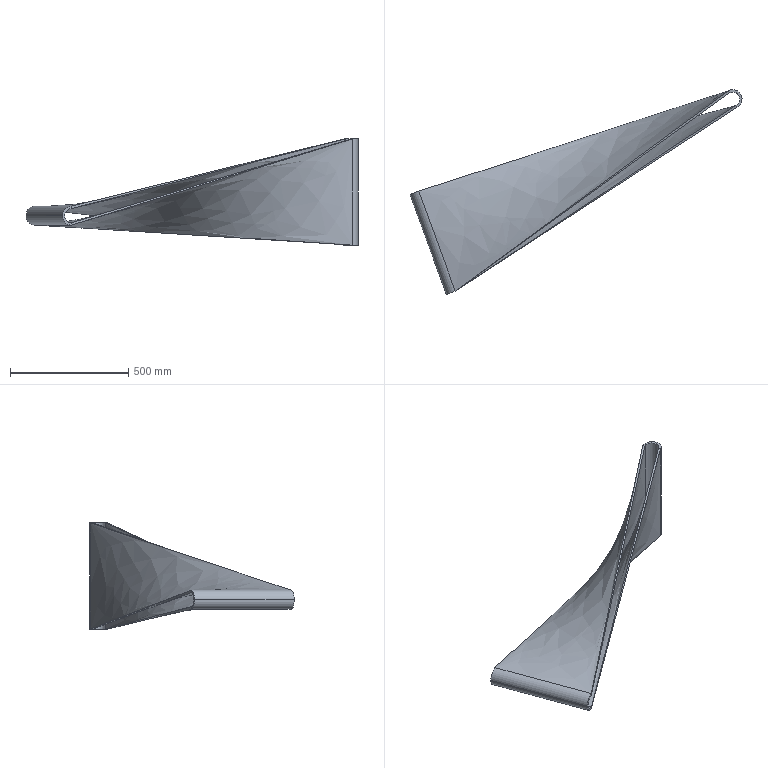Part | SolidWorks | features Blend 2, BossThin 1, ExtruThin 1 | 1 solid | 18 faces | box 1406 x 865.848 x 450 mm | volume 9311838 mm3 | spline 8 | cylinder 6 | plane 4 | commonest cylinder face diameters 60 x3 80 x3
STEP:
#1=CARTESIAN_POINT('',(-1208.342,155.833,-70.));
#2=VERTEX_POINT('',#1);
#3=CARTESIAN_POINT('',(-1236.533,145.573,-100.));
#4=VERTEX_POINT('',#3);
#5=CARTESIAN_POINT('',(-1208.342,155.833,-100.));
#6=DIRECTION('',(0.342,-0.9397,0.));
#7=DIRECTION('',(0.9397,0.342,0.));
#8=AXIS2_PLACEMENT_3D('',#5,#6,#7);
#9=CIRCLE('',#8,30.);
#10=EDGE_CURVE('',#2,#4,#9,.T.);
#11=ORIENTED_EDGE('',*,*,#10,.T.);
#12=CARTESIAN_POINT('',(-1390.442,568.434,-100.));
#13=VERTEX_POINT('',#12);
#14=CARTESIAN_POINT('',(-1236.533,145.573,-100.));
#15=DIRECTION('',(-0.342,0.9397,0.));
#16=VECTOR('',#15,1000.);
#17=LINE('',#14,#16);
#18=EDGE_CURVE('',#4,#13,#17,.T.);
#19=ORIENTED_EDGE('',*,*,#18,.T.);
#20=CARTESIAN_POINT('',(-1362.251,578.695,-70.));
#21=VERTEX_POINT('',#20);
#22=CARTESIAN_POINT('',(-1362.251,578.695,-100.));
#23=DIRECTION('',(0.342,-0.9397,0.));
#24=DIRECTION('',(0.9397,0.342,0.));
#25=AXIS2_PLACEMENT_3D('',#22,#23,#24);
#26=CIRCLE('',#25,30.);
#27=EDGE_CURVE('',#21,#13,#26,.T.);
#28=ORIENTED_EDGE('',*,*,#27,.F.);
#29=CARTESIAN_POINT('',(-1309.238,433.043,-70.));
#30=VERTEX_POINT('',#29);
#31=CARTESIAN_POINT('',(-1309.238,433.043,-70.));
#32=CARTESIAN_POINT('',(-1326.909,481.593,-70.));
#33=CARTESIAN_POINT('',(-1344.58,530.144,-70.));
#34=CARTESIAN_POINT('',(-1362.251,578.695,-70.));
#35=B_SPLINE_CURVE_WITH_KNOTS('',3,(#31,#32,#33,#34),.UNSPECIFIED.,.F.,.F.,(4,4),(0.6556,1.),.UNSPECIFIED.);
#36=EDGE_CURVE('',#30,#21,#35,.T.);
#37=ORIENTED_EDGE('',*,*,#36,.F.);
#38=CARTESIAN_POINT('',(-1208.342,155.833,-70.));
#39=DIRECTION('',(-0.342,0.9397,0.));
#40=VECTOR('',#39,1000.);
#41=LINE('',#38,#40);
#42=EDGE_CURVE('',#2,#30,#41,.T.);
#43=ORIENTED_EDGE('',*,*,#42,.F.);
#44=EDGE_LOOP('',(#11,#19,#28,#37,#43));
#45=FACE_OUTER_BOUND('',#44,.T.);
#46=CARTESIAN_POINT('',(-1208.342,155.833,-100.));
#47=DIRECTION('',(-0.342,0.9397,0.));
#48=DIRECTION('',(-0.9397,-0.342,0.));
#49=AXIS2_PLACEMENT_3D('',#46,#47,#48);
#50=CYLINDRICAL_SURFACE('',#49,30.);
#51=ADVANCED_FACE('',(#45),#50,.F.);
#52=CARTESIAN_POINT('',(-1245.93,142.152,-100.));
#53=VERTEX_POINT('',#52);
#54=CARTESIAN_POINT('',(-1208.342,155.833,-140.));
#55=VERTEX_POINT('',#54);
#56=CARTESIAN_POINT('',(-1208.342,155.833,-100.));
#57=DIRECTION('',(0.342,-0.9397,0.));
#58=DIRECTION('',(0.9397,0.342,0.));
#59=AXIS2_PLACEMENT_3D('',#56,#57,#58);
#60=CIRCLE('',#59,40.);
#61=EDGE_CURVE('',#53,#55,#60,.T.);
#62=ORIENTED_EDGE('',*,*,#61,.F.);
#63=CARTESIAN_POINT('',(-1399.839,565.014,-100.));
#64=VERTEX_POINT('',#63);
#65=CARTESIAN_POINT('',(-1245.93,142.152,-100.));
#66=DIRECTION('',(-0.342,0.9397,0.));
#67=VECTOR('',#66,1000.);
#68=LINE('',#65,#67);
#69=EDGE_CURVE('',#53,#64,#68,.T.);
#70=ORIENTED_EDGE('',*,*,#69,.T.);
#71=CARTESIAN_POINT('',(-1362.251,578.695,-140.));
#72=VERTEX_POINT('',#71);
#73=CARTESIAN_POINT('',(-1362.251,578.695,-100.));
#74=DIRECTION('',(0.342,-0.9397,0.));
#75=DIRECTION('',(0.9397,0.342,0.));
#76=AXIS2_PLACEMENT_3D('',#73,#74,#75);
#77=CIRCLE('',#76,40.);
#78=EDGE_CURVE('',#64,#72,#77,.T.);
#79=ORIENTED_EDGE('',*,*,#78,.T.);
#80=CARTESIAN_POINT('',(-1208.342,155.833,-140.));
#81=DIRECTION('',(-0.342,0.9397,0.));
#82=VECTOR('',#81,1000.);
#83=LINE('',#80,#82);
#84=EDGE_CURVE('',#55,#72,#83,.T.);
#85=ORIENTED_EDGE('',*,*,#84,.F.);
#86=EDGE_LOOP('',(#62,#70,#79,#85));
#87=FACE_OUTER_BOUND('',#86,.T.);
#88=CARTESIAN_POINT('',(-1208.342,155.833,-100.));
#89=DIRECTION('',(-0.342,0.9397,0.));
#90=DIRECTION('',(-0.9397,-0.342,0.));
#91=AXIS2_PLACEMENT_3D('',#88,#89,#90);
#92=CYLINDRICAL_SURFACE('',#91,40.);
#93=ADVANCED_FACE('',(#87),#92,.T.);
#94=CARTESIAN_POINT('',(-16.757,931.979,-225.));
#95=VERTEX_POINT('',#94);
#96=CARTESIAN_POINT('',(-51.541,1004.021,-225.));
#97=VERTEX_POINT('',#96);
#98=CARTESIAN_POINT('',(-34.149,968.,-225.));
#99=DIRECTION('',(0.,0.,1.));
#100=DIRECTION('',(1.,0.,0.));
#101=AXIS2_PLACEMENT_3D('',#98,#99,#100);
#102=CIRCLE('',#101,40.);
#103=EDGE_CURVE('',#95,#97,#102,.T.);
#104=ORIENTED_EDGE('',*,*,#103,.T.);
#105=CARTESIAN_POINT('',(-51.541,1004.021,-37.171));
#106=VERTEX_POINT('',#105);
#107=CARTESIAN_POINT('',(-51.541,1004.021,225.));
#108=DIRECTION('',(0.,0.,-1.));
#109=VECTOR('',#108,1000.);
#110=LINE('',#107,#109);
#111=EDGE_CURVE('',#106,#97,#110,.T.);
#112=ORIENTED_EDGE('',*,*,#111,.F.);
#113=CARTESIAN_POINT('',(-51.541,1004.021,225.));
#114=VERTEX_POINT('',#113);
#115=CARTESIAN_POINT('',(-51.541,1004.021,225.));
#116=DIRECTION('',(0.,0.,-1.));
#117=VECTOR('',#116,1000.);
#118=LINE('',#115,#117);
#119=EDGE_CURVE('',#114,#106,#118,.T.);
#120=ORIENTED_EDGE('',*,*,#119,.F.);
#121=CARTESIAN_POINT('',(-16.757,931.979,225.));
#122=VERTEX_POINT('',#121);
#123=CARTESIAN_POINT('',(-34.149,968.,225.));
#124=DIRECTION('',(0.,0.,1.));
#125=DIRECTION('',(1.,0.,0.));
#126=AXIS2_PLACEMENT_3D('',#123,#124,#125);
#127=CIRCLE('',#126,40.);
#128=EDGE_CURVE('',#122,#114,#127,.T.);
#129=ORIENTED_EDGE('',*,*,#128,.F.);
#130=CARTESIAN_POINT('',(-16.757,931.979,225.));
#131=DIRECTION('',(0.,0.,-1.));
#132=VECTOR('',#131,1000.);
#133=LINE('',#130,#132);
#134=EDGE_CURVE('',#122,#95,#133,.T.);
#135=ORIENTED_EDGE('',*,*,#134,.T.);
#136=EDGE_LOOP('',(#104,#112,#120,#129,#135));
#137=FACE_OUTER_BOUND('',#136,.T.);
#138=CARTESIAN_POINT('',(-34.149,968.,225.));
#139=DIRECTION('',(0.,0.,-1.));
#140=DIRECTION('',(-1.,0.,0.));
#141=AXIS2_PLACEMENT_3D('',#138,#139,#140);
#142=CYLINDRICAL_SURFACE('',#141,40.);
#143=ADVANCED_FACE('',(#137),#142,.T.);
#144=CARTESIAN_POINT('',(-21.105,940.984,-225.));
#145=VERTEX_POINT('',#144);
#146=CARTESIAN_POINT('',(-47.193,995.016,-225.));
#147=VERTEX_POINT('',#146);
#148=CARTESIAN_POINT('',(-34.149,968.,-225.));
#149=DIRECTION('',(0.,0.,1.));
#150=DIRECTION('',(1.,0.,0.));
#151=AXIS2_PLACEMENT_3D('',#148,#149,#150);
#152=CIRCLE('',#151,30.);
#153=EDGE_CURVE('',#145,#147,#152,.T.);
#154=ORIENTED_EDGE('',*,*,#153,.F.);
#155=CARTESIAN_POINT('',(-21.105,940.984,225.));
#156=VERTEX_POINT('',#155);
#157=CARTESIAN_POINT('',(-21.105,940.984,225.));
#158=DIRECTION('',(0.,0.,-1.));
#159=VECTOR('',#158,1000.);
#160=LINE('',#157,#159);
#161=EDGE_CURVE('',#156,#145,#160,.T.);
#162=ORIENTED_EDGE('',*,*,#161,.F.);
#163=CARTESIAN_POINT('',(-47.193,995.016,225.));
#164=VERTEX_POINT('',#163);
#165=CARTESIAN_POINT('',(-34.149,968.,225.));
#166=DIRECTION('',(0.,0.,1.));
#167=DIRECTION('',(1.,0.,0.));
#168=AXIS2_PLACEMENT_3D('',#165,#166,#167);
#169=CIRCLE('',#168,30.);
#170=EDGE_CURVE('',#156,#164,#169,.T.);
#171=ORIENTED_EDGE('',*,*,#170,.T.);
#172=CARTESIAN_POINT('',(-47.193,995.016,-27.12));
#173=VERTEX_POINT('',#172);
#174=CARTESIAN_POINT('',(-47.193,995.016,225.));
#175=DIRECTION('',(0.,0.,-1.));
#176=VECTOR('',#175,1000.);
#177=LINE('',#174,#176);
#178=EDGE_CURVE('',#164,#173,#177,.T.);
#179=ORIENTED_EDGE('',*,*,#178,.T.);
#180=CARTESIAN_POINT('',(-47.193,995.016,225.));
#181=DIRECTION('',(0.,0.,-1.));
#182=VECTOR('',#181,1000.);
#183=LINE('',#180,#182);
#184=EDGE_CURVE('',#173,#147,#183,.T.);
#185=ORIENTED_EDGE('',*,*,#184,.T.);
#186=EDGE_LOOP('',(#154,#162,#171,#179,#185));
#187=FACE_OUTER_BOUND('',#186,.T.);
#188=CARTESIAN_POINT('',(-34.149,968.,225.));
#189=DIRECTION('',(0.,0.,-1.));
#190=DIRECTION('',(-1.,0.,0.));
#191=AXIS2_PLACEMENT_3D('',#188,#189,#190);
#192=CYLINDRICAL_SURFACE('',#191,30.);
#193=ADVANCED_FACE('',(#187),#192,.F.);
#194=ORIENTED_EDGE('',*,*,#128,.T.);
#195=CARTESIAN_POINT('',(-51.541,1004.021,225.));
#196=DIRECTION('',(-0.4348,0.9005,0.));
#197=VECTOR('',#196,1000.);
#198=LINE('',#195,#197);
#199=EDGE_CURVE('',#164,#114,#198,.T.);
#200=ORIENTED_EDGE('',*,*,#199,.F.);
#201=ORIENTED_EDGE('',*,*,#170,.F.);
#202=CARTESIAN_POINT('',(-16.757,931.979,225.));
#203=DIRECTION('',(-0.4348,0.9005,0.));
#204=VECTOR('',#203,1000.);
#205=LINE('',#202,#204);
#206=EDGE_CURVE('',#122,#156,#205,.T.);
#207=ORIENTED_EDGE('',*,*,#206,.F.);
#208=EDGE_LOOP('',(#194,#200,#201,#207));
#209=FACE_OUTER_BOUND('',#208,.T.);
#210=CARTESIAN_POINT('',(-34.149,968.,225.));
#211=DIRECTION('',(0.,0.,1.));
#212=DIRECTION('',(1.,0.,0.));
#213=AXIS2_PLACEMENT_3D('',#210,#211,#212);
#214=PLANE('',#213);
#215=ADVANCED_FACE('',(#209),#214,.T.);
#216=ORIENTED_EDGE('',*,*,#103,.F.);
#217=CARTESIAN_POINT('',(-16.757,931.979,-225.));
#218=DIRECTION('',(-0.4348,0.9005,0.));
#219=VECTOR('',#218,1000.);
#220=LINE('',#217,#219);
#221=EDGE_CURVE('',#95,#145,#220,.T.);
#222=ORIENTED_EDGE('',*,*,#221,.T.);
#223=ORIENTED_EDGE('',*,*,#153,.T.);
#224=CARTESIAN_POINT('',(-47.193,995.016,-225.));
#225=DIRECTION('',(-0.4348,0.9005,0.));
#226=VECTOR('',#225,1000.);
#227=LINE('',#224,#226);
#228=EDGE_CURVE('',#147,#97,#227,.T.);
#229=ORIENTED_EDGE('',*,*,#228,.T.);
#230=EDGE_LOOP('',(#216,#222,#223,#229));
#231=FACE_OUTER_BOUND('',#230,.T.);
#232=CARTESIAN_POINT('',(-34.149,968.,-225.));
#233=DIRECTION('',(0.,0.,1.));
#234=DIRECTION('',(1.,0.,0.));
#235=AXIS2_PLACEMENT_3D('',#232,#233,#234);
#236=PLANE('',#235);
#237=ADVANCED_FACE('',(#231),#236,.F.);
#238=ORIENTED_EDGE('',*,*,#228,.F.);
#239=CARTESIAN_POINT('',(-704.722,786.855,-147.5));
#240=DIRECTION('',(-0.9474,-0.2999,0.1117));
#241=VECTOR('',#240,1000.);
#242=LINE('',#239,#241);
#243=EDGE_CURVE('',#147,#21,#242,.T.);
#244=ORIENTED_EDGE('',*,*,#243,.T.);
#245=CARTESIAN_POINT('',(-1362.251,578.695,-60.));
#246=VERTEX_POINT('',#245);
#247=CARTESIAN_POINT('',(-1362.251,578.695,-60.));
#248=DIRECTION('',(0.,0.,-1.));
#249=VECTOR('',#248,1000.);
#250=LINE('',#247,#249);
#251=EDGE_CURVE('',#246,#21,#250,.T.);
#252=ORIENTED_EDGE('',*,*,#251,.F.);
#253=CARTESIAN_POINT('',(-706.896,791.358,-142.5));
#254=DIRECTION('',(0.9444,0.3065,-0.1189));
#255=VECTOR('',#254,1000.);
#256=LINE('',#253,#255);
#257=EDGE_CURVE('',#246,#97,#256,.T.);
#258=ORIENTED_EDGE('',*,*,#257,.T.);
#259=EDGE_LOOP('',(#238,#244,#252,#258));
#260=FACE_OUTER_BOUND('',#259,.T.);
#261=CARTESIAN_POINT('',(-51.541,1004.021,-225.));
#262=CARTESIAN_POINT('',(-1362.251,578.695,-60.));
#263=CARTESIAN_POINT('',(-50.816,1002.52,-225.));
#264=CARTESIAN_POINT('',(-1362.251,578.695,-61.667));
#265=CARTESIAN_POINT('',(-50.092,1001.019,-225.));
#266=CARTESIAN_POINT('',(-1362.251,578.695,-63.333));
#267=CARTESIAN_POINT('',(-48.642,998.018,-225.));
#268=CARTESIAN_POINT('',(-1362.251,578.695,-66.667));
#269=CARTESIAN_POINT('',(-47.918,996.517,-225.));
#270=CARTESIAN_POINT('',(-1362.251,578.695,-68.333));
#271=CARTESIAN_POINT('',(-47.193,995.016,-225.));
#272=CARTESIAN_POINT('',(-1362.251,578.695,-70.));
#273=B_SPLINE_SURFACE_WITH_KNOTS('',3,1,((#261,#262),(#263,#264),(#265,#266),(#267,#268),(#269,#270),(#271,#272)),.UNSPECIFIED.,.F.,.F.,.F.,(4,2,4),(2,2),(0.,0.5,1.),(0.,1.),.UNSPECIFIED.);
#274=ADVANCED_FACE('',(#260),#273,.T.);
#275=ORIENTED_EDGE('',*,*,#178,.F.);
#276=CARTESIAN_POINT('',(-627.768,575.425,77.5));
#277=DIRECTION('',(-0.7938,-0.5737,-0.2017));
#278=VECTOR('',#277,1000.);
#279=LINE('',#276,#278);
#280=EDGE_CURVE('',#164,#2,#279,.T.);
#281=ORIENTED_EDGE('',*,*,#280,.T.);
#282=ORIENTED_EDGE('',*,*,#42,.T.);
#283=ORIENTED_EDGE('',*,*,#36,.T.);
#284=ORIENTED_EDGE('',*,*,#243,.F.);
#285=ORIENTED_EDGE('',*,*,#184,.F.);
#286=EDGE_LOOP('',(#275,#281,#282,#283,#284,#285));
#287=FACE_OUTER_BOUND('',#286,.T.);
#288=CARTESIAN_POINT('',(-47.193,995.016,-225.));
#289=CARTESIAN_POINT('',(-1362.251,578.695,-70.));
#290=CARTESIAN_POINT('',(-47.193,995.016,-150.));
#291=CARTESIAN_POINT('',(-1336.6,508.218,-70.));
#292=CARTESIAN_POINT('',(-47.193,995.016,-75.));
#293=CARTESIAN_POINT('',(-1310.948,437.741,-70.));
#294=CARTESIAN_POINT('',(-47.193,995.016,75.));
#295=CARTESIAN_POINT('',(-1259.645,296.787,-70.));
#296=CARTESIAN_POINT('',(-47.193,995.016,150.));
#297=CARTESIAN_POINT('',(-1233.994,226.31,-70.));
#298=CARTESIAN_POINT('',(-47.193,995.016,225.));
#299=CARTESIAN_POINT('',(-1208.342,155.833,-70.));
#300=B_SPLINE_SURFACE_WITH_KNOTS('',3,1,((#288,#289),(#290,#291),(#292,#293),(#294,#295),(#296,#297),(#298,#299)),.UNSPECIFIED.,.F.,.F.,.F.,(4,2,4),(2,2),(0.,0.5,1.),(0.,1.),.UNSPECIFIED.);
#301=ADVANCED_FACE('',(#287),#300,.T.);
#302=ORIENTED_EDGE('',*,*,#119,.T.);
#303=ORIENTED_EDGE('',*,*,#111,.T.);
#304=ORIENTED_EDGE('',*,*,#257,.F.);
#305=CARTESIAN_POINT('',(-1305.818,423.646,-60.));
#306=VERTEX_POINT('',#305);
#307=CARTESIAN_POINT('',(-1305.818,423.646,-60.));
#308=CARTESIAN_POINT('',(-1324.629,475.329,-60.));
#309=CARTESIAN_POINT('',(-1343.44,527.012,-60.));
#310=CARTESIAN_POINT('',(-1362.251,578.695,-60.));
#311=B_SPLINE_CURVE_WITH_KNOTS('',3,(#307,#308,#309,#310),.UNSPECIFIED.,.F.,.F.,(4,4),(0.,1.),.UNSPECIFIED.);
#312=EDGE_CURVE('',#306,#246,#311,.T.);
#313=ORIENTED_EDGE('',*,*,#312,.F.);
#314=CARTESIAN_POINT('',(-1208.342,155.833,-60.));
#315=VERTEX_POINT('',#314);
#316=CARTESIAN_POINT('',(-1208.342,155.833,-60.));
#317=DIRECTION('',(-0.342,0.9397,0.));
#318=VECTOR('',#317,1000.);
#319=LINE('',#316,#318);
#320=EDGE_CURVE('',#315,#306,#319,.T.);
#321=ORIENTED_EDGE('',*,*,#320,.F.);
#322=CARTESIAN_POINT('',(-629.942,579.927,82.5));
#323=DIRECTION('',(-0.791,-0.58,-0.1949));
#324=VECTOR('',#323,1000.);
#325=LINE('',#322,#324);
#326=EDGE_CURVE('',#114,#315,#325,.T.);
#327=ORIENTED_EDGE('',*,*,#326,.F.);
#328=EDGE_LOOP('',(#302,#303,#304,#313,#321,#327));
#329=FACE_OUTER_BOUND('',#328,.T.);
#330=CARTESIAN_POINT('',(-51.541,1004.021,225.));
#331=CARTESIAN_POINT('',(-1208.342,155.833,-60.));
#332=CARTESIAN_POINT('',(-51.541,1004.021,150.));
#333=CARTESIAN_POINT('',(-1233.994,226.31,-60.));
#334=CARTESIAN_POINT('',(-51.541,1004.021,75.));
#335=CARTESIAN_POINT('',(-1259.645,296.787,-60.));
#336=CARTESIAN_POINT('',(-51.541,1004.021,-75.));
#337=CARTESIAN_POINT('',(-1310.948,437.741,-60.));
#338=CARTESIAN_POINT('',(-51.541,1004.021,-150.));
#339=CARTESIAN_POINT('',(-1336.6,508.218,-60.));
#340=CARTESIAN_POINT('',(-51.541,1004.021,-225.));
#341=CARTESIAN_POINT('',(-1362.251,578.695,-60.));
#342=B_SPLINE_SURFACE_WITH_KNOTS('',3,1,((#330,#331),(#332,#333),(#334,#335),(#336,#337),(#338,#339),(#340,#341)),.UNSPECIFIED.,.F.,.F.,.F.,(4,2,4),(2,2),(0.,0.5,1.),(0.,1.),.UNSPECIFIED.);
#343=ADVANCED_FACE('',(#329),#342,.T.);
#344=ORIENTED_EDGE('',*,*,#199,.T.);
#345=ORIENTED_EDGE('',*,*,#326,.T.);
#346=CARTESIAN_POINT('',(-1208.342,155.833,-60.));
#347=DIRECTION('',(0.,0.,-1.));
#348=VECTOR('',#347,1000.);
#349=LINE('',#346,#348);
#350=EDGE_CURVE('',#315,#2,#349,.T.);
#351=ORIENTED_EDGE('',*,*,#350,.T.);
#352=ORIENTED_EDGE('',*,*,#280,.F.);
#353=EDGE_LOOP('',(#344,#345,#351,#352));
#354=FACE_OUTER_BOUND('',#353,.T.);
#355=CARTESIAN_POINT('',(-47.193,995.016,225.));
#356=CARTESIAN_POINT('',(-1208.342,155.833,-70.));
#357=CARTESIAN_POINT('',(-47.918,996.517,225.));
#358=CARTESIAN_POINT('',(-1208.342,155.833,-68.333));
#359=CARTESIAN_POINT('',(-48.642,998.018,225.));
#360=CARTESIAN_POINT('',(-1208.342,155.833,-66.667));
#361=CARTESIAN_POINT('',(-50.092,1001.019,225.));
#362=CARTESIAN_POINT('',(-1208.342,155.833,-63.333));
#363=CARTESIAN_POINT('',(-50.816,1002.52,225.));
#364=CARTESIAN_POINT('',(-1208.342,155.833,-61.667));
#365=CARTESIAN_POINT('',(-51.541,1004.021,225.));
#366=CARTESIAN_POINT('',(-1208.342,155.833,-60.));
#367=B_SPLINE_SURFACE_WITH_KNOTS('',3,1,((#355,#356),(#357,#358),(#359,#360),(#361,#362),(#363,#364),(#365,#366)),.UNSPECIFIED.,.F.,.F.,.F.,(4,2,4),(2,2),(0.,0.5,1.),(0.,1.),.UNSPECIFIED.);
#368=ADVANCED_FACE('',(#354),#367,.T.);
#369=ORIENTED_EDGE('',*,*,#69,.F.);
#370=CARTESIAN_POINT('',(-1208.342,155.833,-100.));
#371=DIRECTION('',(0.342,-0.9397,0.));
#372=DIRECTION('',(0.9397,0.342,0.));
#373=AXIS2_PLACEMENT_3D('',#370,#371,#372);
#374=CIRCLE('',#373,40.);
#375=EDGE_CURVE('',#315,#53,#374,.T.);
#376=ORIENTED_EDGE('',*,*,#375,.F.);
#377=ORIENTED_EDGE('',*,*,#320,.T.);
#378=ORIENTED_EDGE('',*,*,#312,.T.);
#379=CARTESIAN_POINT('',(-1362.251,578.695,-100.));
#380=DIRECTION('',(0.342,-0.9397,0.));
#381=DIRECTION('',(0.9397,0.342,0.));
#382=AXIS2_PLACEMENT_3D('',#379,#380,#381);
#383=CIRCLE('',#382,40.);
#384=EDGE_CURVE('',#246,#64,#383,.T.);
#385=ORIENTED_EDGE('',*,*,#384,.T.);
#386=EDGE_LOOP('',(#369,#376,#377,#378,#385));
#387=FACE_OUTER_BOUND('',#386,.T.);
#388=CARTESIAN_POINT('',(-1208.342,155.833,-100.));
#389=DIRECTION('',(-0.342,0.9397,0.));
#390=DIRECTION('',(-0.9397,-0.342,0.));
#391=AXIS2_PLACEMENT_3D('',#388,#389,#390);
#392=CYLINDRICAL_SURFACE('',#391,40.);
#393=ADVANCED_FACE('',(#387),#392,.T.);
#394=ORIENTED_EDGE('',*,*,#18,.F.);
#395=CARTESIAN_POINT('',(-1208.342,155.833,-130.));
#396=VERTEX_POINT('',#395);
#397=CARTESIAN_POINT('',(-1208.342,155.833,-100.));
#398=DIRECTION('',(0.342,-0.9397,0.));
#399=DIRECTION('',(0.9397,0.342,0.));
#400=AXIS2_PLACEMENT_3D('',#397,#398,#399);
#401=CIRCLE('',#400,30.);
#402=EDGE_CURVE('',#4,#396,#401,.T.);
#403=ORIENTED_EDGE('',*,*,#402,.T.);
#404=CARTESIAN_POINT('',(-1362.251,578.695,-130.));
#405=VERTEX_POINT('',#404);
#406=CARTESIAN_POINT('',(-1208.342,155.833,-130.));
#407=DIRECTION('',(-0.342,0.9397,0.));
#408=VECTOR('',#407,1000.);
#409=LINE('',#406,#408);
#410=EDGE_CURVE('',#396,#405,#409,.T.);
#411=ORIENTED_EDGE('',*,*,#410,.T.);
#412=CARTESIAN_POINT('',(-1362.251,578.695,-100.));
#413=DIRECTION('',(0.342,-0.9397,0.));
#414=DIRECTION('',(0.9397,0.342,0.));
#415=AXIS2_PLACEMENT_3D('',#412,#413,#414);
#416=CIRCLE('',#415,30.);
#417=EDGE_CURVE('',#13,#405,#416,.T.);
#418=ORIENTED_EDGE('',*,*,#417,.F.);
#419=EDGE_LOOP('',(#394,#403,#411,#418));
#420=FACE_OUTER_BOUND('',#419,.T.);
#421=CARTESIAN_POINT('',(-1208.342,155.833,-100.));
#422=DIRECTION('',(-0.342,0.9397,0.));
#423=DIRECTION('',(-0.9397,-0.342,0.));
#424=AXIS2_PLACEMENT_3D('',#421,#422,#423);
#425=CYLINDRICAL_SURFACE('',#424,30.);
#426=ADVANCED_FACE('',(#420),#425,.F.);
#427=ORIENTED_EDGE('',*,*,#375,.T.);
#428=ORIENTED_EDGE('',*,*,#61,.T.);
#429=CARTESIAN_POINT('',(-1208.342,155.833,-130.));
#430=DIRECTION('',(0.,0.,-1.));
#431=VECTOR('',#430,1000.);
#432=LINE('',#429,#431);
#433=EDGE_CURVE('',#396,#55,#432,.T.);
#434=ORIENTED_EDGE('',*,*,#433,.F.);
#435=ORIENTED_EDGE('',*,*,#402,.F.);
#436=ORIENTED_EDGE('',*,*,#10,.F.);
#437=ORIENTED_EDGE('',*,*,#350,.F.);
#438=EDGE_LOOP('',(#427,#428,#434,#435,#436,#437));
#439=FACE_OUTER_BOUND('',#438,.T.);
#440=CARTESIAN_POINT('',(-1208.342,155.833,-100.));
#441=DIRECTION('',(0.342,-0.9397,0.));
#442=DIRECTION('',(0.9397,0.342,0.));
#443=AXIS2_PLACEMENT_3D('',#440,#441,#442);
#444=PLANE('',#443);
#445=ADVANCED_FACE('',(#439),#444,.T.);
#446=ORIENTED_EDGE('',*,*,#384,.F.);
#447=ORIENTED_EDGE('',*,*,#251,.T.);
#448=ORIENTED_EDGE('',*,*,#27,.T.);
#449=ORIENTED_EDGE('',*,*,#417,.T.);
#450=CARTESIAN_POINT('',(-1362.251,578.695,-130.));
#451=DIRECTION('',(0.,0.,-1.));
#452=VECTOR('',#451,1000.);
#453=LINE('',#450,#452);
#454=EDGE_CURVE('',#405,#72,#453,.T.);
#455=ORIENTED_EDGE('',*,*,#454,.T.);
#456=ORIENTED_EDGE('',*,*,#78,.F.);
#457=EDGE_LOOP('',(#446,#447,#448,#449,#455,#456));
#458=FACE_OUTER_BOUND('',#457,.T.);
#459=CARTESIAN_POINT('',(-1362.251,578.695,-100.));
#460=DIRECTION('',(0.342,-0.9397,0.));
#461=DIRECTION('',(0.9397,0.342,0.));
#462=AXIS2_PLACEMENT_3D('',#459,#460,#461);
#463=PLANE('',#462);
#464=ADVANCED_FACE('',(#458),#463,.F.);
#465=ORIENTED_EDGE('',*,*,#134,.F.);
#466=CARTESIAN_POINT('',(-612.55,543.906,42.5));
#467=DIRECTION('',(-0.8116,-0.5287,-0.2486));
#468=VECTOR('',#467,1000.);
#469=LINE('',#466,#468);
#470=EDGE_CURVE('',#122,#55,#469,.T.);
#471=ORIENTED_EDGE('',*,*,#470,.T.);
#472=ORIENTED_EDGE('',*,*,#84,.T.);
#473=CARTESIAN_POINT('',(-689.504,755.337,-182.5));
#474=DIRECTION('',(0.9654,0.2535,-0.06099));
#475=VECTOR('',#474,1000.);
#476=LINE('',#473,#475);
#477=EDGE_CURVE('',#72,#95,#476,.T.);
#478=ORIENTED_EDGE('',*,*,#477,.T.);
#479=EDGE_LOOP('',(#465,#471,#472,#478));
#480=FACE_OUTER_BOUND('',#479,.T.);
#481=CARTESIAN_POINT('',(-16.757,931.979,-225.));
#482=CARTESIAN_POINT('',(-1362.251,578.695,-140.));
#483=CARTESIAN_POINT('',(-16.757,931.979,-150.));
#484=CARTESIAN_POINT('',(-1336.6,508.218,-140.));
#485=CARTESIAN_POINT('',(-16.757,931.979,-75.));
#486=CARTESIAN_POINT('',(-1310.948,437.741,-140.));
#487=CARTESIAN_POINT('',(-16.757,931.979,75.));
#488=CARTESIAN_POINT('',(-1259.645,296.787,-140.));
#489=CARTESIAN_POINT('',(-16.757,931.979,150.));
#490=CARTESIAN_POINT('',(-1233.994,226.31,-140.));
#491=CARTESIAN_POINT('',(-16.757,931.979,225.));
#492=CARTESIAN_POINT('',(-1208.342,155.833,-140.));
#493=B_SPLINE_SURFACE_WITH_KNOTS('',3,1,((#481,#482),(#483,#484),(#485,#486),(#487,#488),(#489,#490),(#491,#492)),.UNSPECIFIED.,.F.,.F.,.F.,(4,2,4),(2,2),(0.,0.5,1.),(0.,1.),.UNSPECIFIED.);
#494=ADVANCED_FACE('',(#480),#493,.T.);
#495=ORIENTED_EDGE('',*,*,#206,.T.);
#496=CARTESIAN_POINT('',(-614.724,548.409,47.5));
#497=DIRECTION('',(-0.8093,-0.5352,-0.242));
#498=VECTOR('',#497,1000.);
#499=LINE('',#496,#498);
#500=EDGE_CURVE('',#156,#396,#499,.T.);
#501=ORIENTED_EDGE('',*,*,#500,.T.);
#502=ORIENTED_EDGE('',*,*,#433,.T.);
#503=ORIENTED_EDGE('',*,*,#470,.F.);
#504=EDGE_LOOP('',(#495,#501,#502,#503));
#505=FACE_OUTER_BOUND('',#504,.T.);
#506=CARTESIAN_POINT('',(-16.757,931.979,225.));
#507=CARTESIAN_POINT('',(-1208.342,155.833,-140.));
#508=CARTESIAN_POINT('',(-17.482,933.48,225.));
#509=CARTESIAN_POINT('',(-1208.342,155.833,-138.333));
#510=CARTESIAN_POINT('',(-18.206,934.981,225.));
#511=CARTESIAN_POINT('',(-1208.342,155.833,-136.667));
#512=CARTESIAN_POINT('',(-19.656,937.982,225.));
#513=CARTESIAN_POINT('',(-1208.342,155.833,-133.333));
#514=CARTESIAN_POINT('',(-20.38,939.483,225.));
#515=CARTESIAN_POINT('',(-1208.342,155.833,-131.667));
#516=CARTESIAN_POINT('',(-21.105,940.984,225.));
#517=CARTESIAN_POINT('',(-1208.342,155.833,-130.));
#518=B_SPLINE_SURFACE_WITH_KNOTS('',3,1,((#506,#507),(#508,#509),(#510,#511),(#512,#513),(#514,#515),(#516,#517)),.UNSPECIFIED.,.F.,.F.,.F.,(4,2,4),(2,2),(0.,0.5,1.),(0.,1.),.UNSPECIFIED.);
#519=ADVANCED_FACE('',(#505),#518,.T.);
#520=ORIENTED_EDGE('',*,*,#221,.F.);
#521=ORIENTED_EDGE('',*,*,#477,.F.);
#522=ORIENTED_EDGE('',*,*,#454,.F.);
#523=CARTESIAN_POINT('',(-691.678,759.84,-177.5));
#524=DIRECTION('',(-0.9631,-0.2602,0.06822));
#525=VECTOR('',#524,1000.);
#526=LINE('',#523,#525);
#527=EDGE_CURVE('',#145,#405,#526,.T.);
#528=ORIENTED_EDGE('',*,*,#527,.F.);
#529=EDGE_LOOP('',(#520,#521,#522,#528));
#530=FACE_OUTER_BOUND('',#529,.T.);
#531=CARTESIAN_POINT('',(-21.105,940.984,-225.));
#532=CARTESIAN_POINT('',(-1362.251,578.695,-130.));
#533=CARTESIAN_POINT('',(-20.38,939.483,-225.));
#534=CARTESIAN_POINT('',(-1362.251,578.695,-131.667));
#535=CARTESIAN_POINT('',(-19.656,937.982,-225.));
#536=CARTESIAN_POINT('',(-1362.251,578.695,-133.333));
#537=CARTESIAN_POINT('',(-18.206,934.981,-225.));
#538=CARTESIAN_POINT('',(-1362.251,578.695,-136.667));
#539=CARTESIAN_POINT('',(-17.482,933.48,-225.));
#540=CARTESIAN_POINT('',(-1362.251,578.695,-138.333));
#541=CARTESIAN_POINT('',(-16.757,931.979,-225.));
#542=CARTESIAN_POINT('',(-1362.251,578.695,-140.));
#543=B_SPLINE_SURFACE_WITH_KNOTS('',3,1,((#531,#532),(#533,#534),(#535,#536),(#537,#538),(#539,#540),(#541,#542)),.UNSPECIFIED.,.F.,.F.,.F.,(4,2,4),(2,2),(0.,0.5,1.),(0.,1.),.UNSPECIFIED.);
#544=ADVANCED_FACE('',(#530),#543,.T.);
#545=ORIENTED_EDGE('',*,*,#161,.T.);
#546=ORIENTED_EDGE('',*,*,#527,.T.);
#547=ORIENTED_EDGE('',*,*,#410,.F.);
#548=ORIENTED_EDGE('',*,*,#500,.F.);
#549=EDGE_LOOP('',(#545,#546,#547,#548));
#550=FACE_OUTER_BOUND('',#549,.T.);
#551=CARTESIAN_POINT('',(-21.105,940.984,225.));
#552=CARTESIAN_POINT('',(-1208.342,155.833,-130.));
#553=CARTESIAN_POINT('',(-21.105,940.984,150.));
#554=CARTESIAN_POINT('',(-1233.994,226.31,-130.));
#555=CARTESIAN_POINT('',(-21.105,940.984,75.));
#556=CARTESIAN_POINT('',(-1259.645,296.787,-130.));
#557=CARTESIAN_POINT('',(-21.105,940.984,-75.));
#558=CARTESIAN_POINT('',(-1310.948,437.741,-130.));
#559=CARTESIAN_POINT('',(-21.105,940.984,-150.));
#560=CARTESIAN_POINT('',(-1336.6,508.218,-130.));
#561=CARTESIAN_POINT('',(-21.105,940.984,-225.));
#562=CARTESIAN_POINT('',(-1362.251,578.695,-130.));
#563=B_SPLINE_SURFACE_WITH_KNOTS('',3,1,((#551,#552),(#553,#554),(#555,#556),(#557,#558),(#559,#560),(#561,#562)),.UNSPECIFIED.,.F.,.F.,.F.,(4,2,4),(2,2),(0.,0.5,1.),(0.,1.),.UNSPECIFIED.);
#564=ADVANCED_FACE('',(#550),#563,.T.);
#565=CLOSED_SHELL('',(#51,#93,#143,#193,#215,#237,#274,#301,#343,#368,#393,#426,#445,#464,#494,#519,#544,#564));
#566=MANIFOLD_SOLID_BREP('',#565);
#567=CARTESIAN_POINT('',(0.,0.,0.));
#568=DIRECTION('',(0.,0.,1.));
#569=DIRECTION('',(1.,0.,0.));
#570=AXIS2_PLACEMENT_3D('',#567,#568,#569);
#571=(LENGTH_UNIT()NAMED_UNIT(*)SI_UNIT(.MILLI.,.METRE.));
#572=UNCERTAINTY_MEASURE_WITH_UNIT(LENGTH_MEASURE(0.00001),#571,'','');
#573=(NAMED_UNIT(*)PLANE_ANGLE_UNIT()SI_UNIT($,.RADIAN.));
#574=(NAMED_UNIT(*)SI_UNIT($,.STERADIAN.)SOLID_ANGLE_UNIT());
#575=(GEOMETRIC_REPRESENTATION_CONTEXT(3)GLOBAL_UNCERTAINTY_ASSIGNED_CONTEXT((#572))GLOBAL_UNIT_ASSIGNED_CONTEXT((#571,#573,#574))REPRESENTATION_CONTEXT('',''));
#576=ADVANCED_BREP_SHAPE_REPRESENTATION('',(#566,#570),#575);